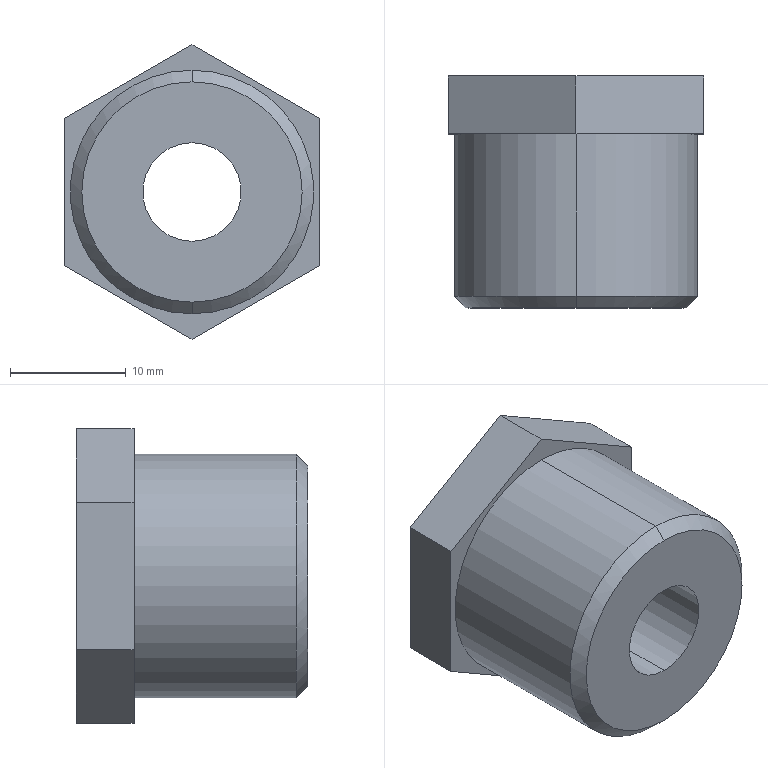Part | SolidWorks | features 3DProfileFeature 1, Chamfer 1, Extrusion 1, HoleWzd 1, ICE 1 | 1 solid | 15 faces | box 22 x 20 x 25.403 mm | volume 6124 mm3 | plane 9 | cylinder 4 | cone 2 | commonest cylinder face diameters 8.5 x2 21 x2
STEP:
#1=CARTESIAN_POINT('',(0.,0.,-4.25));
#2=VERTEX_POINT('',#1);
#3=CARTESIAN_POINT('',(0.,0.,4.25));
#4=VERTEX_POINT('',#3);
#5=CARTESIAN_POINT('',(0.,0.,0.));
#6=DIRECTION('',(0.,1.,0.));
#7=DIRECTION('',(0.,0.,1.));
#8=AXIS2_PLACEMENT_3D('',#5,#6,#7);
#9=CIRCLE('',#8,4.25);
#10=EDGE_CURVE('',#2,#4,#9,.T.);
#11=ORIENTED_EDGE('',*,*,#10,.F.);
#12=CARTESIAN_POINT('',(0.,20.,-4.25));
#13=VERTEX_POINT('',#12);
#14=CARTESIAN_POINT('',(0.,20.,-4.25));
#15=DIRECTION('',(0.,1.,0.));
#16=VECTOR('',#15,1000.);
#17=LINE('',#14,#16);
#18=EDGE_CURVE('',#2,#13,#17,.T.);
#19=ORIENTED_EDGE('',*,*,#18,.T.);
#20=CARTESIAN_POINT('',(0.,20.,4.25));
#21=VERTEX_POINT('',#20);
#22=CARTESIAN_POINT('',(0.,20.,0.));
#23=DIRECTION('',(0.,1.,0.));
#24=DIRECTION('',(0.,0.,1.));
#25=AXIS2_PLACEMENT_3D('',#22,#23,#24);
#26=CIRCLE('',#25,4.25);
#27=EDGE_CURVE('',#13,#21,#26,.T.);
#28=ORIENTED_EDGE('',*,*,#27,.T.);
#29=CARTESIAN_POINT('',(0.,20.,4.25));
#30=DIRECTION('',(0.,1.,0.));
#31=VECTOR('',#30,1000.);
#32=LINE('',#29,#31);
#33=EDGE_CURVE('',#4,#21,#32,.T.);
#34=ORIENTED_EDGE('',*,*,#33,.F.);
#35=EDGE_LOOP('',(#11,#19,#28,#34));
#36=FACE_OUTER_BOUND('',#35,.T.);
#37=CARTESIAN_POINT('',(0.,20.,0.));
#38=DIRECTION('',(0.,1.,0.));
#39=DIRECTION('',(0.,0.,1.));
#40=AXIS2_PLACEMENT_3D('',#37,#38,#39);
#41=CYLINDRICAL_SURFACE('',#40,4.25);
#42=ADVANCED_FACE('',(#36),#41,.F.);
#43=CARTESIAN_POINT('',(0.,0.,-9.5));
#44=VERTEX_POINT('',#43);
#45=CARTESIAN_POINT('',(0.,0.,9.5));
#46=VERTEX_POINT('',#45);
#47=CARTESIAN_POINT('',(0.,0.,0.));
#48=DIRECTION('',(0.,-1.,0.));
#49=DIRECTION('',(0.,0.,1.));
#50=AXIS2_PLACEMENT_3D('',#47,#48,#49);
#51=CIRCLE('',#50,9.5);
#52=EDGE_CURVE('',#44,#46,#51,.T.);
#53=ORIENTED_EDGE('',*,*,#52,.F.);
#54=CARTESIAN_POINT('',(0.,1.,-10.5));
#55=VERTEX_POINT('',#54);
#56=CARTESIAN_POINT('',(0.,0.,-9.5));
#57=DIRECTION('',(0.,0.7071,-0.7071));
#58=VECTOR('',#57,1000.);
#59=LINE('',#56,#58);
#60=EDGE_CURVE('',#44,#55,#59,.T.);
#61=ORIENTED_EDGE('',*,*,#60,.T.);
#62=CARTESIAN_POINT('',(0.,1.,10.5));
#63=VERTEX_POINT('',#62);
#64=CARTESIAN_POINT('',(0.,1.,0.));
#65=DIRECTION('',(0.,1.,0.));
#66=DIRECTION('',(0.,0.,1.));
#67=AXIS2_PLACEMENT_3D('',#64,#65,#66);
#68=CIRCLE('',#67,10.5);
#69=EDGE_CURVE('',#63,#55,#68,.T.);
#70=ORIENTED_EDGE('',*,*,#69,.F.);
#71=CARTESIAN_POINT('',(0.,0.,9.5));
#72=DIRECTION('',(0.,0.7071,0.7071));
#73=VECTOR('',#72,1000.);
#74=LINE('',#71,#73);
#75=EDGE_CURVE('',#46,#63,#74,.T.);
#76=ORIENTED_EDGE('',*,*,#75,.F.);
#77=EDGE_LOOP('',(#53,#61,#70,#76));
#78=FACE_OUTER_BOUND('',#77,.T.);
#79=CARTESIAN_POINT('',(0.,0.,0.));
#80=DIRECTION('',(0.,1.,0.));
#81=DIRECTION('',(0.,0.,1.));
#82=AXIS2_PLACEMENT_3D('',#79,#80,#81);
#83=CONICAL_SURFACE('',#82,9.5,0.7854);
#84=ADVANCED_FACE('',(#78),#83,.T.);
#85=CARTESIAN_POINT('',(0.,15.,-10.5));
#86=VERTEX_POINT('',#85);
#87=CARTESIAN_POINT('',(0.,15.,10.5));
#88=VERTEX_POINT('',#87);
#89=CARTESIAN_POINT('',(0.,15.,0.));
#90=DIRECTION('',(0.,-1.,0.));
#91=DIRECTION('',(0.,0.,1.));
#92=AXIS2_PLACEMENT_3D('',#89,#90,#91);
#93=CIRCLE('',#92,10.5);
#94=EDGE_CURVE('',#86,#88,#93,.T.);
#95=ORIENTED_EDGE('',*,*,#94,.T.);
#96=CARTESIAN_POINT('',(0.,53.942,10.5));
#97=DIRECTION('',(0.,-1.,0.));
#98=VECTOR('',#97,1000.);
#99=LINE('',#96,#98);
#100=EDGE_CURVE('',#88,#63,#99,.T.);
#101=ORIENTED_EDGE('',*,*,#100,.T.);
#102=ORIENTED_EDGE('',*,*,#69,.T.);
#103=CARTESIAN_POINT('',(0.,53.942,-10.5));
#104=DIRECTION('',(0.,-1.,0.));
#105=VECTOR('',#104,1000.);
#106=LINE('',#103,#105);
#107=EDGE_CURVE('',#86,#55,#106,.T.);
#108=ORIENTED_EDGE('',*,*,#107,.F.);
#109=EDGE_LOOP('',(#95,#101,#102,#108));
#110=FACE_OUTER_BOUND('',#109,.T.);
#111=CARTESIAN_POINT('',(0.,53.942,0.));
#112=DIRECTION('',(0.,-1.,0.));
#113=DIRECTION('',(0.,0.,-1.));
#114=AXIS2_PLACEMENT_3D('',#111,#112,#113);
#115=CYLINDRICAL_SURFACE('',#114,10.5);
#116=ADVANCED_FACE('',(#110),#115,.T.);
#117=CARTESIAN_POINT('',(0.,20.,12.702));
#118=VERTEX_POINT('',#117);
#119=CARTESIAN_POINT('',(0.,15.,12.702));
#120=VERTEX_POINT('',#119);
#121=CARTESIAN_POINT('',(0.,20.,12.702));
#122=DIRECTION('',(0.,-1.,0.));
#123=VECTOR('',#122,1000.);
#124=LINE('',#121,#123);
#125=EDGE_CURVE('',#118,#120,#124,.T.);
#126=ORIENTED_EDGE('',*,*,#125,.T.);
#127=CARTESIAN_POINT('',(11.,15.,6.351));
#128=VERTEX_POINT('',#127);
#129=CARTESIAN_POINT('',(0.,15.,12.702));
#130=DIRECTION('',(0.866,0.,-0.5));
#131=VECTOR('',#130,1000.);
#132=LINE('',#129,#131);
#133=EDGE_CURVE('',#120,#128,#132,.T.);
#134=ORIENTED_EDGE('',*,*,#133,.T.);
#135=CARTESIAN_POINT('',(11.,20.,6.351));
#136=VERTEX_POINT('',#135);
#137=CARTESIAN_POINT('',(11.,20.,6.351));
#138=DIRECTION('',(0.,-1.,0.));
#139=VECTOR('',#138,1000.);
#140=LINE('',#137,#139);
#141=EDGE_CURVE('',#136,#128,#140,.T.);
#142=ORIENTED_EDGE('',*,*,#141,.F.);
#143=CARTESIAN_POINT('',(0.,20.,12.702));
#144=DIRECTION('',(0.866,0.,-0.5));
#145=VECTOR('',#144,1000.);
#146=LINE('',#143,#145);
#147=EDGE_CURVE('',#118,#136,#146,.T.);
#148=ORIENTED_EDGE('',*,*,#147,.F.);
#149=EDGE_LOOP('',(#126,#134,#142,#148));
#150=FACE_OUTER_BOUND('',#149,.T.);
#151=CARTESIAN_POINT('',(0.,20.,12.702));
#152=DIRECTION('',(-0.5,0.,-0.866));
#153=DIRECTION('',(-0.866,0.,0.5));
#154=AXIS2_PLACEMENT_3D('',#151,#152,#153);
#155=PLANE('',#154);
#156=ADVANCED_FACE('',(#150),#155,.F.);
#157=ORIENTED_EDGE('',*,*,#141,.T.);
#158=CARTESIAN_POINT('',(11.,15.,-6.351));
#159=VERTEX_POINT('',#158);
#160=CARTESIAN_POINT('',(11.,15.,6.351));
#161=DIRECTION('',(0.,0.,-1.));
#162=VECTOR('',#161,1000.);
#163=LINE('',#160,#162);
#164=EDGE_CURVE('',#128,#159,#163,.T.);
#165=ORIENTED_EDGE('',*,*,#164,.T.);
#166=CARTESIAN_POINT('',(11.,20.,-6.351));
#167=VERTEX_POINT('',#166);
#168=CARTESIAN_POINT('',(11.,20.,-6.351));
#169=DIRECTION('',(0.,-1.,0.));
#170=VECTOR('',#169,1000.);
#171=LINE('',#168,#170);
#172=EDGE_CURVE('',#167,#159,#171,.T.);
#173=ORIENTED_EDGE('',*,*,#172,.F.);
#174=CARTESIAN_POINT('',(11.,20.,6.351));
#175=DIRECTION('',(0.,0.,-1.));
#176=VECTOR('',#175,1000.);
#177=LINE('',#174,#176);
#178=EDGE_CURVE('',#136,#167,#177,.T.);
#179=ORIENTED_EDGE('',*,*,#178,.F.);
#180=EDGE_LOOP('',(#157,#165,#173,#179));
#181=FACE_OUTER_BOUND('',#180,.T.);
#182=CARTESIAN_POINT('',(11.,20.,6.351));
#183=DIRECTION('',(-1.,0.,0.));
#184=DIRECTION('',(0.,0.,1.));
#185=AXIS2_PLACEMENT_3D('',#182,#183,#184);
#186=PLANE('',#185);
#187=ADVANCED_FACE('',(#181),#186,.F.);
#188=ORIENTED_EDGE('',*,*,#172,.T.);
#189=CARTESIAN_POINT('',(0.,15.,-12.702));
#190=VERTEX_POINT('',#189);
#191=CARTESIAN_POINT('',(11.,15.,-6.351));
#192=DIRECTION('',(-0.866,0.,-0.5));
#193=VECTOR('',#192,1000.);
#194=LINE('',#191,#193);
#195=EDGE_CURVE('',#159,#190,#194,.T.);
#196=ORIENTED_EDGE('',*,*,#195,.T.);
#197=CARTESIAN_POINT('',(0.,20.,-12.702));
#198=VERTEX_POINT('',#197);
#199=CARTESIAN_POINT('',(0.,20.,-12.702));
#200=DIRECTION('',(0.,-1.,0.));
#201=VECTOR('',#200,1000.);
#202=LINE('',#199,#201);
#203=EDGE_CURVE('',#198,#190,#202,.T.);
#204=ORIENTED_EDGE('',*,*,#203,.F.);
#205=CARTESIAN_POINT('',(11.,20.,-6.351));
#206=DIRECTION('',(-0.866,0.,-0.5));
#207=VECTOR('',#206,1000.);
#208=LINE('',#205,#207);
#209=EDGE_CURVE('',#167,#198,#208,.T.);
#210=ORIENTED_EDGE('',*,*,#209,.F.);
#211=EDGE_LOOP('',(#188,#196,#204,#210));
#212=FACE_OUTER_BOUND('',#211,.T.);
#213=CARTESIAN_POINT('',(11.,20.,-6.351));
#214=DIRECTION('',(-0.5,0.,0.866));
#215=DIRECTION('',(0.866,0.,0.5));
#216=AXIS2_PLACEMENT_3D('',#213,#214,#215);
#217=PLANE('',#216);
#218=ADVANCED_FACE('',(#212),#217,.F.);
#219=ORIENTED_EDGE('',*,*,#203,.T.);
#220=CARTESIAN_POINT('',(-11.,15.,-6.351));
#221=VERTEX_POINT('',#220);
#222=CARTESIAN_POINT('',(0.,15.,-12.702));
#223=DIRECTION('',(-0.866,0.,0.5));
#224=VECTOR('',#223,1000.);
#225=LINE('',#222,#224);
#226=EDGE_CURVE('',#190,#221,#225,.T.);
#227=ORIENTED_EDGE('',*,*,#226,.T.);
#228=CARTESIAN_POINT('',(-11.,20.,-6.351));
#229=VERTEX_POINT('',#228);
#230=CARTESIAN_POINT('',(-11.,20.,-6.351));
#231=DIRECTION('',(0.,-1.,0.));
#232=VECTOR('',#231,1000.);
#233=LINE('',#230,#232);
#234=EDGE_CURVE('',#229,#221,#233,.T.);
#235=ORIENTED_EDGE('',*,*,#234,.F.);
#236=CARTESIAN_POINT('',(0.,20.,-12.702));
#237=DIRECTION('',(-0.866,0.,0.5));
#238=VECTOR('',#237,1000.);
#239=LINE('',#236,#238);
#240=EDGE_CURVE('',#198,#229,#239,.T.);
#241=ORIENTED_EDGE('',*,*,#240,.F.);
#242=EDGE_LOOP('',(#219,#227,#235,#241));
#243=FACE_OUTER_BOUND('',#242,.T.);
#244=CARTESIAN_POINT('',(0.,20.,-12.702));
#245=DIRECTION('',(0.5,0.,0.866));
#246=DIRECTION('',(0.866,0.,-0.5));
#247=AXIS2_PLACEMENT_3D('',#244,#245,#246);
#248=PLANE('',#247);
#249=ADVANCED_FACE('',(#243),#248,.F.);
#250=ORIENTED_EDGE('',*,*,#234,.T.);
#251=CARTESIAN_POINT('',(-11.,15.,6.351));
#252=VERTEX_POINT('',#251);
#253=CARTESIAN_POINT('',(-11.,15.,-6.351));
#254=DIRECTION('',(0.,0.,1.));
#255=VECTOR('',#254,1000.);
#256=LINE('',#253,#255);
#257=EDGE_CURVE('',#221,#252,#256,.T.);
#258=ORIENTED_EDGE('',*,*,#257,.T.);
#259=CARTESIAN_POINT('',(-11.,20.,6.351));
#260=VERTEX_POINT('',#259);
#261=CARTESIAN_POINT('',(-11.,20.,6.351));
#262=DIRECTION('',(0.,-1.,0.));
#263=VECTOR('',#262,1000.);
#264=LINE('',#261,#263);
#265=EDGE_CURVE('',#260,#252,#264,.T.);
#266=ORIENTED_EDGE('',*,*,#265,.F.);
#267=CARTESIAN_POINT('',(-11.,20.,-6.351));
#268=DIRECTION('',(0.,0.,1.));
#269=VECTOR('',#268,1000.);
#270=LINE('',#267,#269);
#271=EDGE_CURVE('',#229,#260,#270,.T.);
#272=ORIENTED_EDGE('',*,*,#271,.F.);
#273=EDGE_LOOP('',(#250,#258,#266,#272));
#274=FACE_OUTER_BOUND('',#273,.T.);
#275=CARTESIAN_POINT('',(-11.,20.,-6.351));
#276=DIRECTION('',(1.,0.,0.));
#277=DIRECTION('',(0.,0.,-1.));
#278=AXIS2_PLACEMENT_3D('',#275,#276,#277);
#279=PLANE('',#278);
#280=ADVANCED_FACE('',(#274),#279,.F.);
#281=ORIENTED_EDGE('',*,*,#265,.T.);
#282=CARTESIAN_POINT('',(-11.,15.,6.351));
#283=DIRECTION('',(0.866,0.,0.5));
#284=VECTOR('',#283,1000.);
#285=LINE('',#282,#284);
#286=EDGE_CURVE('',#252,#120,#285,.T.);
#287=ORIENTED_EDGE('',*,*,#286,.T.);
#288=ORIENTED_EDGE('',*,*,#125,.F.);
#289=CARTESIAN_POINT('',(-11.,20.,6.351));
#290=DIRECTION('',(0.866,0.,0.5));
#291=VECTOR('',#290,1000.);
#292=LINE('',#289,#291);
#293=EDGE_CURVE('',#260,#118,#292,.T.);
#294=ORIENTED_EDGE('',*,*,#293,.F.);
#295=EDGE_LOOP('',(#281,#287,#288,#294));
#296=FACE_OUTER_BOUND('',#295,.T.);
#297=CARTESIAN_POINT('',(-11.,20.,6.351));
#298=DIRECTION('',(0.5,0.,-0.866));
#299=DIRECTION('',(-0.866,0.,-0.5));
#300=AXIS2_PLACEMENT_3D('',#297,#298,#299);
#301=PLANE('',#300);
#302=ADVANCED_FACE('',(#296),#301,.F.);
#303=CARTESIAN_POINT('',(0.,20.,0.));
#304=DIRECTION('',(0.,1.,0.));
#305=DIRECTION('',(0.,0.,1.));
#306=AXIS2_PLACEMENT_3D('',#303,#304,#305);
#307=CIRCLE('',#306,4.25);
#308=EDGE_CURVE('',#21,#13,#307,.T.);
#309=ORIENTED_EDGE('',*,*,#308,.F.);
#310=ORIENTED_EDGE('',*,*,#27,.F.);
#311=EDGE_LOOP('',(#309,#310));
#312=FACE_BOUND('',#311,.T.);
#313=ORIENTED_EDGE('',*,*,#147,.T.);
#314=ORIENTED_EDGE('',*,*,#178,.T.);
#315=ORIENTED_EDGE('',*,*,#209,.T.);
#316=ORIENTED_EDGE('',*,*,#240,.T.);
#317=ORIENTED_EDGE('',*,*,#271,.T.);
#318=ORIENTED_EDGE('',*,*,#293,.T.);
#319=EDGE_LOOP('',(#313,#314,#315,#316,#317,#318));
#320=FACE_OUTER_BOUND('',#319,.T.);
#321=CARTESIAN_POINT('',(0.,20.,0.));
#322=DIRECTION('',(0.,1.,0.));
#323=DIRECTION('',(0.,0.,1.));
#324=AXIS2_PLACEMENT_3D('',#321,#322,#323);
#325=PLANE('',#324);
#326=ADVANCED_FACE('',(#312,#320),#325,.T.);
#327=ORIENTED_EDGE('',*,*,#94,.F.);
#328=CARTESIAN_POINT('',(0.,15.,0.));
#329=DIRECTION('',(0.,-1.,0.));
#330=DIRECTION('',(0.,0.,1.));
#331=AXIS2_PLACEMENT_3D('',#328,#329,#330);
#332=CIRCLE('',#331,10.5);
#333=EDGE_CURVE('',#88,#86,#332,.T.);
#334=ORIENTED_EDGE('',*,*,#333,.F.);
#335=EDGE_LOOP('',(#327,#334));
#336=FACE_BOUND('',#335,.T.);
#337=ORIENTED_EDGE('',*,*,#286,.F.);
#338=ORIENTED_EDGE('',*,*,#257,.F.);
#339=ORIENTED_EDGE('',*,*,#226,.F.);
#340=ORIENTED_EDGE('',*,*,#195,.F.);
#341=ORIENTED_EDGE('',*,*,#164,.F.);
#342=ORIENTED_EDGE('',*,*,#133,.F.);
#343=EDGE_LOOP('',(#337,#338,#339,#340,#341,#342));
#344=FACE_OUTER_BOUND('',#343,.T.);
#345=CARTESIAN_POINT('',(0.,15.,0.));
#346=DIRECTION('',(0.,1.,0.));
#347=DIRECTION('',(0.,0.,1.));
#348=AXIS2_PLACEMENT_3D('',#345,#346,#347);
#349=PLANE('',#348);
#350=ADVANCED_FACE('',(#336,#344),#349,.F.);
#351=ORIENTED_EDGE('',*,*,#100,.F.);
#352=ORIENTED_EDGE('',*,*,#333,.T.);
#353=ORIENTED_EDGE('',*,*,#107,.T.);
#354=CARTESIAN_POINT('',(0.,1.,0.));
#355=DIRECTION('',(0.,1.,0.));
#356=DIRECTION('',(0.,0.,1.));
#357=AXIS2_PLACEMENT_3D('',#354,#355,#356);
#358=CIRCLE('',#357,10.5);
#359=EDGE_CURVE('',#55,#63,#358,.T.);
#360=ORIENTED_EDGE('',*,*,#359,.T.);
#361=EDGE_LOOP('',(#351,#352,#353,#360));
#362=FACE_OUTER_BOUND('',#361,.T.);
#363=CARTESIAN_POINT('',(0.,53.942,0.));
#364=DIRECTION('',(0.,-1.,0.));
#365=DIRECTION('',(0.,0.,-1.));
#366=AXIS2_PLACEMENT_3D('',#363,#364,#365);
#367=CYLINDRICAL_SURFACE('',#366,10.5);
#368=ADVANCED_FACE('',(#362),#367,.T.);
#369=CARTESIAN_POINT('',(0.,0.,0.));
#370=DIRECTION('',(0.,1.,0.));
#371=DIRECTION('',(0.,0.,1.));
#372=AXIS2_PLACEMENT_3D('',#369,#370,#371);
#373=CIRCLE('',#372,4.25);
#374=EDGE_CURVE('',#4,#2,#373,.T.);
#375=ORIENTED_EDGE('',*,*,#374,.T.);
#376=ORIENTED_EDGE('',*,*,#10,.T.);
#377=EDGE_LOOP('',(#375,#376));
#378=FACE_BOUND('',#377,.T.);
#379=CARTESIAN_POINT('',(0.,0.,0.));
#380=DIRECTION('',(0.,-1.,0.));
#381=DIRECTION('',(0.,0.,1.));
#382=AXIS2_PLACEMENT_3D('',#379,#380,#381);
#383=CIRCLE('',#382,9.5);
#384=EDGE_CURVE('',#46,#44,#383,.T.);
#385=ORIENTED_EDGE('',*,*,#384,.T.);
#386=ORIENTED_EDGE('',*,*,#52,.T.);
#387=EDGE_LOOP('',(#385,#386));
#388=FACE_OUTER_BOUND('',#387,.T.);
#389=CARTESIAN_POINT('',(0.,0.,0.));
#390=DIRECTION('',(0.,1.,0.));
#391=DIRECTION('',(0.,0.,1.));
#392=AXIS2_PLACEMENT_3D('',#389,#390,#391);
#393=PLANE('',#392);
#394=ADVANCED_FACE('',(#378,#388),#393,.F.);
#395=ORIENTED_EDGE('',*,*,#60,.F.);
#396=ORIENTED_EDGE('',*,*,#384,.F.);
#397=ORIENTED_EDGE('',*,*,#75,.T.);
#398=ORIENTED_EDGE('',*,*,#359,.F.);
#399=EDGE_LOOP('',(#395,#396,#397,#398));
#400=FACE_OUTER_BOUND('',#399,.T.);
#401=CARTESIAN_POINT('',(0.,0.,0.));
#402=DIRECTION('',(0.,1.,0.));
#403=DIRECTION('',(0.,0.,1.));
#404=AXIS2_PLACEMENT_3D('',#401,#402,#403);
#405=CONICAL_SURFACE('',#404,9.5,0.7854);
#406=ADVANCED_FACE('',(#400),#405,.T.);
#407=ORIENTED_EDGE('',*,*,#18,.F.);
#408=ORIENTED_EDGE('',*,*,#374,.F.);
#409=ORIENTED_EDGE('',*,*,#33,.T.);
#410=ORIENTED_EDGE('',*,*,#308,.T.);
#411=EDGE_LOOP('',(#407,#408,#409,#410));
#412=FACE_OUTER_BOUND('',#411,.T.);
#413=CARTESIAN_POINT('',(0.,20.,0.));
#414=DIRECTION('',(0.,1.,0.));
#415=DIRECTION('',(0.,0.,1.));
#416=AXIS2_PLACEMENT_3D('',#413,#414,#415);
#417=CYLINDRICAL_SURFACE('',#416,4.25);
#418=ADVANCED_FACE('',(#412),#417,.F.);
#419=CLOSED_SHELL('',(#42,#84,#116,#156,#187,#218,#249,#280,#302,#326,#350,#368,#394,#406,#418));
#420=MANIFOLD_SOLID_BREP('',#419);
#421=CARTESIAN_POINT('',(0.,0.,0.));
#422=DIRECTION('',(0.,0.,1.));
#423=DIRECTION('',(1.,0.,0.));
#424=AXIS2_PLACEMENT_3D('',#421,#422,#423);
#425=(LENGTH_UNIT()NAMED_UNIT(*)SI_UNIT(.MILLI.,.METRE.));
#426=UNCERTAINTY_MEASURE_WITH_UNIT(LENGTH_MEASURE(0.00001),#425,'','');
#427=(NAMED_UNIT(*)PLANE_ANGLE_UNIT()SI_UNIT($,.RADIAN.));
#428=(NAMED_UNIT(*)SI_UNIT($,.STERADIAN.)SOLID_ANGLE_UNIT());
#429=(GEOMETRIC_REPRESENTATION_CONTEXT(3)GLOBAL_UNCERTAINTY_ASSIGNED_CONTEXT((#426))GLOBAL_UNIT_ASSIGNED_CONTEXT((#425,#427,#428))REPRESENTATION_CONTEXT('',''));
#430=ADVANCED_BREP_SHAPE_REPRESENTATION('',(#420,#424),#429);